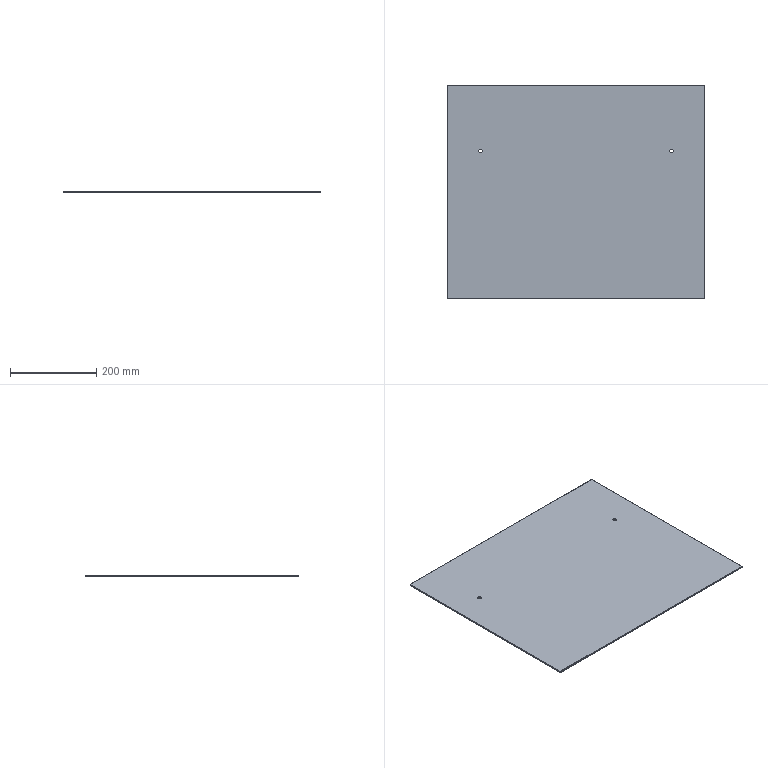Part | STEP file | ZXW722-L-05 | 1 solid | 22 faces | box 596 x 494 x 3 mm | volume 882649 mm3 | plane 10 | cylinder 8 | cone 4 | commonest cylinder face diameters 4 x4 8.5 x4
STEP:
#1=CARTESIAN_POINT('',(0.,0.,0.));
#2=DIRECTION('',(0.,0.,1.));
#3=DIRECTION('',(1.,0.,0.));
#4=AXIS2_PLACEMENT_3D('',#1,#2,#3);
#5=CARTESIAN_POINT('',(296.,245.5,0.000000011));
#6=VERTEX_POINT('',#5);
#7=CARTESIAN_POINT('',(-296.,245.5,0.));
#8=VERTEX_POINT('',#7);
#9=CARTESIAN_POINT('',(296.,245.5,0.000000011));
#10=DIRECTION('',(-1.,0.,0.));
#11=VECTOR('',#10,592.);
#12=LINE('',#9,#11);
#13=EDGE_CURVE('',#6,#8,#12,.T.);
#14=ORIENTED_EDGE('',*,*,#13,.F.);
#15=CARTESIAN_POINT('',(297.5,244.,0.));
#16=VERTEX_POINT('',#15);
#17=CARTESIAN_POINT('',(296.,244.,0.));
#18=DIRECTION('',(0.,0.,1.));
#19=DIRECTION('',(1.,0.,0.));
#20=AXIS2_PLACEMENT_3D('',#17,#18,#19);
#21=CIRCLE('',#20,1.5);
#22=EDGE_CURVE('',#16,#6,#21,.T.);
#23=ORIENTED_EDGE('',*,*,#22,.F.);
#24=CARTESIAN_POINT('',(297.5,-246.,0.));
#25=VERTEX_POINT('',#24);
#26=CARTESIAN_POINT('',(297.5,-246.,0.000000011));
#27=DIRECTION('',(0.,1.,0.));
#28=VECTOR('',#27,490.);
#29=LINE('',#26,#28);
#30=EDGE_CURVE('',#25,#16,#29,.T.);
#31=ORIENTED_EDGE('',*,*,#30,.F.);
#32=CARTESIAN_POINT('',(296.,-247.5,0.));
#33=VERTEX_POINT('',#32);
#34=CARTESIAN_POINT('',(296.,-246.,0.));
#35=DIRECTION('',(0.,0.,1.));
#36=DIRECTION('',(0.,-1.,0.));
#37=AXIS2_PLACEMENT_3D('',#34,#35,#36);
#38=CIRCLE('',#37,1.5);
#39=EDGE_CURVE('',#33,#25,#38,.T.);
#40=ORIENTED_EDGE('',*,*,#39,.F.);
#41=CARTESIAN_POINT('',(-296.,-247.5,0.));
#42=VERTEX_POINT('',#41);
#43=CARTESIAN_POINT('',(-296.,-247.5,0.000000011));
#44=DIRECTION('',(1.,0.,0.));
#45=VECTOR('',#44,592.);
#46=LINE('',#43,#45);
#47=EDGE_CURVE('',#42,#33,#46,.T.);
#48=ORIENTED_EDGE('',*,*,#47,.F.);
#49=CARTESIAN_POINT('',(-297.5,-246.,0.));
#50=VERTEX_POINT('',#49);
#51=CARTESIAN_POINT('',(-296.,-246.,0.));
#52=DIRECTION('',(0.,0.,1.));
#53=DIRECTION('',(-1.,0.,0.));
#54=AXIS2_PLACEMENT_3D('',#51,#52,#53);
#55=CIRCLE('',#54,1.5);
#56=EDGE_CURVE('',#50,#42,#55,.T.);
#57=ORIENTED_EDGE('',*,*,#56,.F.);
#58=CARTESIAN_POINT('',(-297.5,244.,0.));
#59=VERTEX_POINT('',#58);
#60=CARTESIAN_POINT('',(-297.5,244.,0.000000011));
#61=DIRECTION('',(0.,-1.,0.));
#62=VECTOR('',#61,490.);
#63=LINE('',#60,#62);
#64=EDGE_CURVE('',#59,#50,#63,.T.);
#65=ORIENTED_EDGE('',*,*,#64,.F.);
#66=CARTESIAN_POINT('',(-296.,244.,0.));
#67=DIRECTION('',(0.,0.,1.));
#68=DIRECTION('',(0.,1.,0.));
#69=AXIS2_PLACEMENT_3D('',#66,#67,#68);
#70=CIRCLE('',#69,1.5);
#71=EDGE_CURVE('',#8,#59,#70,.T.);
#72=ORIENTED_EDGE('',*,*,#71,.F.);
#73=EDGE_LOOP('',(#14,#23,#31,#40,#48,#57,#65,#72));
#74=FACE_OUTER_BOUND('',#73,.F.);
#75=CARTESIAN_POINT('',(-217.25,94.,0.));
#76=VERTEX_POINT('',#75);
#77=CARTESIAN_POINT('',(-225.75,94.,0.));
#78=VERTEX_POINT('',#77);
#79=CARTESIAN_POINT('',(-221.5,94.,0.));
#80=DIRECTION('',(0.,0.,1.));
#81=DIRECTION('',(1.,0.,0.));
#82=AXIS2_PLACEMENT_3D('',#79,#80,#81);
#83=CIRCLE('',#82,4.25);
#84=EDGE_CURVE('',#76,#78,#83,.T.);
#85=ORIENTED_EDGE('',*,*,#84,.T.);
#86=CARTESIAN_POINT('',(-221.5,94.,0.));
#87=DIRECTION('',(0.,0.,1.));
#88=DIRECTION('',(-1.,0.,0.));
#89=AXIS2_PLACEMENT_3D('',#86,#87,#88);
#90=CIRCLE('',#89,4.25);
#91=EDGE_CURVE('',#78,#76,#90,.T.);
#92=ORIENTED_EDGE('',*,*,#91,.T.);
#93=EDGE_LOOP('',(#85,#92));
#94=FACE_BOUND('',#93,.F.);
#95=CARTESIAN_POINT('',(225.75,94.,0.));
#96=VERTEX_POINT('',#95);
#97=CARTESIAN_POINT('',(217.25,94.,0.));
#98=VERTEX_POINT('',#97);
#99=CARTESIAN_POINT('',(221.5,94.,0.));
#100=DIRECTION('',(0.,0.,1.));
#101=DIRECTION('',(1.,0.,0.));
#102=AXIS2_PLACEMENT_3D('',#99,#100,#101);
#103=CIRCLE('',#102,4.25);
#104=EDGE_CURVE('',#96,#98,#103,.T.);
#105=ORIENTED_EDGE('',*,*,#104,.T.);
#106=CARTESIAN_POINT('',(221.5,94.,0.));
#107=DIRECTION('',(0.,0.,1.));
#108=DIRECTION('',(-1.,0.,0.));
#109=AXIS2_PLACEMENT_3D('',#106,#107,#108);
#110=CIRCLE('',#109,4.25);
#111=EDGE_CURVE('',#98,#96,#110,.T.);
#112=ORIENTED_EDGE('',*,*,#111,.T.);
#113=EDGE_LOOP('',(#105,#112));
#114=FACE_BOUND('',#113,.F.);
#115=CARTESIAN_POINT('',(0.,0.,0.));
#116=DIRECTION('',(0.,0.,1.));
#117=DIRECTION('',(1.,0.,0.));
#118=AXIS2_PLACEMENT_3D('',#115,#116,#117);
#119=PLANE('',#118);
#120=ADVANCED_FACE('',(#74,#94,#114),#119,.T.);
#121=ORIENTED_EDGE('',*,*,#13,.T.);
#122=CARTESIAN_POINT('',(-296.,246.,-0.5));
#123=VERTEX_POINT('',#122);
#124=CARTESIAN_POINT('',(-296.,245.5,0.));
#125=DIRECTION('',(0.,0.7071,-0.7071));
#126=VECTOR('',#125,0.7071);
#127=LINE('',#124,#126);
#128=EDGE_CURVE('',#8,#123,#127,.T.);
#129=ORIENTED_EDGE('',*,*,#128,.T.);
#130=CARTESIAN_POINT('',(296.,246.,-0.5));
#131=VERTEX_POINT('',#130);
#132=CARTESIAN_POINT('',(296.,246.,-0.5));
#133=DIRECTION('',(-1.,0.,0.));
#134=VECTOR('',#133,592.);
#135=LINE('',#132,#134);
#136=EDGE_CURVE('',#131,#123,#135,.T.);
#137=ORIENTED_EDGE('',*,*,#136,.F.);
#138=CARTESIAN_POINT('',(296.,245.5,0.000000011));
#139=DIRECTION('',(0.,0.7071,-0.7071));
#140=VECTOR('',#139,0.7071);
#141=LINE('',#138,#140);
#142=EDGE_CURVE('',#6,#131,#141,.T.);
#143=ORIENTED_EDGE('',*,*,#142,.F.);
#144=EDGE_LOOP('',(#121,#129,#137,#143));
#145=FACE_OUTER_BOUND('',#144,.F.);
#146=CARTESIAN_POINT('',(0.,245.75,-0.25));
#147=DIRECTION('',(0.,0.7071,0.7071));
#148=DIRECTION('',(0.,0.7071,-0.7071));
#149=AXIS2_PLACEMENT_3D('',#146,#147,#148);
#150=PLANE('',#149);
#151=ADVANCED_FACE('',(#145),#150,.T.);
#152=ORIENTED_EDGE('',*,*,#71,.T.);
#153=CARTESIAN_POINT('',(-298.,244.,-0.5));
#154=VERTEX_POINT('',#153);
#155=CARTESIAN_POINT('',(-297.5,244.,0.000000011));
#156=DIRECTION('',(-0.7071,0.,-0.7071));
#157=VECTOR('',#156,0.7071);
#158=LINE('',#155,#157);
#159=EDGE_CURVE('',#59,#154,#158,.T.);
#160=ORIENTED_EDGE('',*,*,#159,.T.);
#161=CARTESIAN_POINT('',(-296.,244.,-0.5));
#162=DIRECTION('',(0.,0.,1.));
#163=DIRECTION('',(0.,1.,0.));
#164=AXIS2_PLACEMENT_3D('',#161,#162,#163);
#165=CIRCLE('',#164,2.);
#166=EDGE_CURVE('',#123,#154,#165,.T.);
#167=ORIENTED_EDGE('',*,*,#166,.F.);
#168=ORIENTED_EDGE('',*,*,#128,.F.);
#169=EDGE_LOOP('',(#152,#160,#167,#168));
#170=FACE_OUTER_BOUND('',#169,.F.);
#171=CARTESIAN_POINT('',(-296.,244.,-0.25));
#172=DIRECTION('',(0.,0.,-1.));
#173=DIRECTION('',(0.,-1.,0.));
#174=AXIS2_PLACEMENT_3D('',#171,#172,#173);
#175=CONICAL_SURFACE('',#174,1.75,45.);
#176=ADVANCED_FACE('',(#170),#175,.T.);
#177=ORIENTED_EDGE('',*,*,#64,.T.);
#178=CARTESIAN_POINT('',(-298.,-246.,-0.5));
#179=VERTEX_POINT('',#178);
#180=CARTESIAN_POINT('',(-297.5,-246.,0.));
#181=DIRECTION('',(-0.7071,0.,-0.7071));
#182=VECTOR('',#181,0.7071);
#183=LINE('',#180,#182);
#184=EDGE_CURVE('',#50,#179,#183,.T.);
#185=ORIENTED_EDGE('',*,*,#184,.T.);
#186=CARTESIAN_POINT('',(-298.,244.,-0.5));
#187=DIRECTION('',(0.,-1.,0.));
#188=VECTOR('',#187,490.);
#189=LINE('',#186,#188);
#190=EDGE_CURVE('',#154,#179,#189,.T.);
#191=ORIENTED_EDGE('',*,*,#190,.F.);
#192=ORIENTED_EDGE('',*,*,#159,.F.);
#193=EDGE_LOOP('',(#177,#185,#191,#192));
#194=FACE_OUTER_BOUND('',#193,.F.);
#195=CARTESIAN_POINT('',(-297.75,-1.,-0.25));
#196=DIRECTION('',(-0.7071,0.,0.7071));
#197=DIRECTION('',(-0.7071,0.,-0.7071));
#198=AXIS2_PLACEMENT_3D('',#195,#196,#197);
#199=PLANE('',#198);
#200=ADVANCED_FACE('',(#194),#199,.T.);
#201=ORIENTED_EDGE('',*,*,#56,.T.);
#202=CARTESIAN_POINT('',(-296.,-248.,-0.5));
#203=VERTEX_POINT('',#202);
#204=CARTESIAN_POINT('',(-296.,-247.5,0.000000011));
#205=DIRECTION('',(0.,-0.7071,-0.7071));
#206=VECTOR('',#205,0.7071);
#207=LINE('',#204,#206);
#208=EDGE_CURVE('',#42,#203,#207,.T.);
#209=ORIENTED_EDGE('',*,*,#208,.T.);
#210=CARTESIAN_POINT('',(-296.,-246.,-0.5));
#211=DIRECTION('',(0.,0.,1.));
#212=DIRECTION('',(-1.,0.,0.));
#213=AXIS2_PLACEMENT_3D('',#210,#211,#212);
#214=CIRCLE('',#213,2.);
#215=EDGE_CURVE('',#179,#203,#214,.T.);
#216=ORIENTED_EDGE('',*,*,#215,.F.);
#217=ORIENTED_EDGE('',*,*,#184,.F.);
#218=EDGE_LOOP('',(#201,#209,#216,#217));
#219=FACE_OUTER_BOUND('',#218,.F.);
#220=CARTESIAN_POINT('',(-296.,-246.,-0.25));
#221=DIRECTION('',(0.,0.,-1.));
#222=DIRECTION('',(0.,-1.,0.));
#223=AXIS2_PLACEMENT_3D('',#220,#221,#222);
#224=CONICAL_SURFACE('',#223,1.75,45.);
#225=ADVANCED_FACE('',(#219),#224,.T.);
#226=ORIENTED_EDGE('',*,*,#47,.T.);
#227=CARTESIAN_POINT('',(296.,-248.,-0.5));
#228=VERTEX_POINT('',#227);
#229=CARTESIAN_POINT('',(296.,-247.5,0.));
#230=DIRECTION('',(0.,-0.7071,-0.7071));
#231=VECTOR('',#230,0.7071);
#232=LINE('',#229,#231);
#233=EDGE_CURVE('',#33,#228,#232,.T.);
#234=ORIENTED_EDGE('',*,*,#233,.T.);
#235=CARTESIAN_POINT('',(-296.,-248.,-0.5));
#236=DIRECTION('',(1.,0.,0.));
#237=VECTOR('',#236,592.);
#238=LINE('',#235,#237);
#239=EDGE_CURVE('',#203,#228,#238,.T.);
#240=ORIENTED_EDGE('',*,*,#239,.F.);
#241=ORIENTED_EDGE('',*,*,#208,.F.);
#242=EDGE_LOOP('',(#226,#234,#240,#241));
#243=FACE_OUTER_BOUND('',#242,.F.);
#244=CARTESIAN_POINT('',(0.,-247.75,-0.25));
#245=DIRECTION('',(0.,-0.7071,0.7071));
#246=DIRECTION('',(0.,-0.7071,-0.7071));
#247=AXIS2_PLACEMENT_3D('',#244,#245,#246);
#248=PLANE('',#247);
#249=ADVANCED_FACE('',(#243),#248,.T.);
#250=ORIENTED_EDGE('',*,*,#39,.T.);
#251=CARTESIAN_POINT('',(298.,-246.,-0.5));
#252=VERTEX_POINT('',#251);
#253=CARTESIAN_POINT('',(297.5,-246.,0.000000011));
#254=DIRECTION('',(0.7071,0.,-0.7071));
#255=VECTOR('',#254,0.7071);
#256=LINE('',#253,#255);
#257=EDGE_CURVE('',#25,#252,#256,.T.);
#258=ORIENTED_EDGE('',*,*,#257,.T.);
#259=CARTESIAN_POINT('',(296.,-246.,-0.5));
#260=DIRECTION('',(0.,0.,1.));
#261=DIRECTION('',(0.,-1.,0.));
#262=AXIS2_PLACEMENT_3D('',#259,#260,#261);
#263=CIRCLE('',#262,2.);
#264=EDGE_CURVE('',#228,#252,#263,.T.);
#265=ORIENTED_EDGE('',*,*,#264,.F.);
#266=ORIENTED_EDGE('',*,*,#233,.F.);
#267=EDGE_LOOP('',(#250,#258,#265,#266));
#268=FACE_OUTER_BOUND('',#267,.F.);
#269=CARTESIAN_POINT('',(296.,-246.,-0.25));
#270=DIRECTION('',(0.,0.,-1.));
#271=DIRECTION('',(0.,-1.,0.));
#272=AXIS2_PLACEMENT_3D('',#269,#270,#271);
#273=CONICAL_SURFACE('',#272,1.75,45.);
#274=ADVANCED_FACE('',(#268),#273,.T.);
#275=ORIENTED_EDGE('',*,*,#30,.T.);
#276=CARTESIAN_POINT('',(298.,244.,-0.5));
#277=VERTEX_POINT('',#276);
#278=CARTESIAN_POINT('',(297.5,244.,0.));
#279=DIRECTION('',(0.7071,0.,-0.7071));
#280=VECTOR('',#279,0.7071);
#281=LINE('',#278,#280);
#282=EDGE_CURVE('',#16,#277,#281,.T.);
#283=ORIENTED_EDGE('',*,*,#282,.T.);
#284=CARTESIAN_POINT('',(298.,-246.,-0.5));
#285=DIRECTION('',(0.,1.,0.));
#286=VECTOR('',#285,490.);
#287=LINE('',#284,#286);
#288=EDGE_CURVE('',#252,#277,#287,.T.);
#289=ORIENTED_EDGE('',*,*,#288,.F.);
#290=ORIENTED_EDGE('',*,*,#257,.F.);
#291=EDGE_LOOP('',(#275,#283,#289,#290));
#292=FACE_OUTER_BOUND('',#291,.F.);
#293=CARTESIAN_POINT('',(297.75,-1.,-0.25));
#294=DIRECTION('',(0.7071,0.,0.7071));
#295=DIRECTION('',(0.7071,0.,-0.7071));
#296=AXIS2_PLACEMENT_3D('',#293,#294,#295);
#297=PLANE('',#296);
#298=ADVANCED_FACE('',(#292),#297,.T.);
#299=ORIENTED_EDGE('',*,*,#142,.T.);
#300=CARTESIAN_POINT('',(296.,244.,-0.5));
#301=DIRECTION('',(0.,0.,1.));
#302=DIRECTION('',(1.,0.,0.));
#303=AXIS2_PLACEMENT_3D('',#300,#301,#302);
#304=CIRCLE('',#303,2.);
#305=EDGE_CURVE('',#277,#131,#304,.T.);
#306=ORIENTED_EDGE('',*,*,#305,.F.);
#307=ORIENTED_EDGE('',*,*,#282,.F.);
#308=ORIENTED_EDGE('',*,*,#22,.T.);
#309=EDGE_LOOP('',(#299,#306,#307,#308));
#310=FACE_OUTER_BOUND('',#309,.F.);
#311=CARTESIAN_POINT('',(296.,244.,-0.25));
#312=DIRECTION('',(0.,0.,-1.));
#313=DIRECTION('',(0.,-1.,0.));
#314=AXIS2_PLACEMENT_3D('',#311,#312,#313);
#315=CONICAL_SURFACE('',#314,1.75,45.);
#316=ADVANCED_FACE('',(#310),#315,.T.);
#317=ORIENTED_EDGE('',*,*,#305,.T.);
#318=CARTESIAN_POINT('',(296.,246.,-3.));
#319=VERTEX_POINT('',#318);
#320=CARTESIAN_POINT('',(296.,246.,-0.5));
#321=DIRECTION('',(-0.00000002,0.000000004,-1.));
#322=VECTOR('',#321,2.5);
#323=LINE('',#320,#322);
#324=EDGE_CURVE('',#131,#319,#323,.T.);
#325=ORIENTED_EDGE('',*,*,#324,.T.);
#326=CARTESIAN_POINT('',(298.,244.,-3.));
#327=VERTEX_POINT('',#326);
#328=CARTESIAN_POINT('',(296.,244.,-3.));
#329=DIRECTION('',(0.,0.,-1.));
#330=DIRECTION('',(0.,1.,0.));
#331=AXIS2_PLACEMENT_3D('',#328,#329,#330);
#332=CIRCLE('',#331,2.);
#333=EDGE_CURVE('',#319,#327,#332,.T.);
#334=ORIENTED_EDGE('',*,*,#333,.T.);
#335=CARTESIAN_POINT('',(298.,244.,-0.5));
#336=DIRECTION('',(0.,0.,-1.));
#337=VECTOR('',#336,2.5);
#338=LINE('',#335,#337);
#339=EDGE_CURVE('',#277,#327,#338,.T.);
#340=ORIENTED_EDGE('',*,*,#339,.F.);
#341=EDGE_LOOP('',(#317,#325,#334,#340));
#342=FACE_OUTER_BOUND('',#341,.F.);
#343=CARTESIAN_POINT('',(296.,244.,3.911));
#344=DIRECTION('',(0.,0.,-1.));
#345=DIRECTION('',(0.,1.,0.));
#346=AXIS2_PLACEMENT_3D('',#343,#344,#345);
#347=CYLINDRICAL_SURFACE('',#346,2.);
#348=ADVANCED_FACE('',(#342),#347,.T.);
#349=ORIENTED_EDGE('',*,*,#136,.T.);
#350=CARTESIAN_POINT('',(-296.,246.,-3.));
#351=VERTEX_POINT('',#350);
#352=CARTESIAN_POINT('',(-296.,246.,-0.5));
#353=DIRECTION('',(0.,0.,-1.));
#354=VECTOR('',#353,2.5);
#355=LINE('',#352,#354);
#356=EDGE_CURVE('',#123,#351,#355,.T.);
#357=ORIENTED_EDGE('',*,*,#356,.T.);
#358=CARTESIAN_POINT('',(296.,246.,-3.));
#359=DIRECTION('',(-1.,0.,0.));
#360=VECTOR('',#359,592.);
#361=LINE('',#358,#360);
#362=EDGE_CURVE('',#319,#351,#361,.T.);
#363=ORIENTED_EDGE('',*,*,#362,.F.);
#364=ORIENTED_EDGE('',*,*,#324,.F.);
#365=EDGE_LOOP('',(#349,#357,#363,#364));
#366=FACE_OUTER_BOUND('',#365,.F.);
#367=CARTESIAN_POINT('',(297.5,246.,0.));
#368=DIRECTION('',(0.,1.,0.));
#369=DIRECTION('',(-1.,0.,0.));
#370=AXIS2_PLACEMENT_3D('',#367,#368,#369);
#371=PLANE('',#370);
#372=ADVANCED_FACE('',(#366),#371,.T.);
#373=ORIENTED_EDGE('',*,*,#166,.T.);
#374=CARTESIAN_POINT('',(-298.,244.,-3.));
#375=VERTEX_POINT('',#374);
#376=CARTESIAN_POINT('',(-298.,244.,-0.5));
#377=DIRECTION('',(-0.000000004,-0.00000002,-1.));
#378=VECTOR('',#377,2.5);
#379=LINE('',#376,#378);
#380=EDGE_CURVE('',#154,#375,#379,.T.);
#381=ORIENTED_EDGE('',*,*,#380,.T.);
#382=CARTESIAN_POINT('',(-296.,244.,-3.));
#383=DIRECTION('',(0.,0.,-1.));
#384=DIRECTION('',(-1.,0.,0.));
#385=AXIS2_PLACEMENT_3D('',#382,#383,#384);
#386=CIRCLE('',#385,2.);
#387=EDGE_CURVE('',#375,#351,#386,.T.);
#388=ORIENTED_EDGE('',*,*,#387,.T.);
#389=ORIENTED_EDGE('',*,*,#356,.F.);
#390=EDGE_LOOP('',(#373,#381,#388,#389));
#391=FACE_OUTER_BOUND('',#390,.F.);
#392=CARTESIAN_POINT('',(-296.,244.,3.911));
#393=DIRECTION('',(0.,0.,-1.));
#394=DIRECTION('',(-1.,0.,0.));
#395=AXIS2_PLACEMENT_3D('',#392,#393,#394);
#396=CYLINDRICAL_SURFACE('',#395,2.);
#397=ADVANCED_FACE('',(#391),#396,.T.);
#398=ORIENTED_EDGE('',*,*,#190,.T.);
#399=CARTESIAN_POINT('',(-298.,-246.,-3.));
#400=VERTEX_POINT('',#399);
#401=CARTESIAN_POINT('',(-298.,-246.,-0.5));
#402=DIRECTION('',(0.,0.,-1.));
#403=VECTOR('',#402,2.5);
#404=LINE('',#401,#403);
#405=EDGE_CURVE('',#179,#400,#404,.T.);
#406=ORIENTED_EDGE('',*,*,#405,.T.);
#407=CARTESIAN_POINT('',(-298.,244.,-3.));
#408=DIRECTION('',(0.,-1.,0.));
#409=VECTOR('',#408,490.);
#410=LINE('',#407,#409);
#411=EDGE_CURVE('',#375,#400,#410,.T.);
#412=ORIENTED_EDGE('',*,*,#411,.F.);
#413=ORIENTED_EDGE('',*,*,#380,.F.);
#414=EDGE_LOOP('',(#398,#406,#412,#413));
#415=FACE_OUTER_BOUND('',#414,.F.);
#416=CARTESIAN_POINT('',(-298.,246.,0.));
#417=DIRECTION('',(-1.,0.,0.));
#418=DIRECTION('',(0.,-1.,0.));
#419=AXIS2_PLACEMENT_3D('',#416,#417,#418);
#420=PLANE('',#419);
#421=ADVANCED_FACE('',(#415),#420,.T.);
#422=ORIENTED_EDGE('',*,*,#215,.T.);
#423=CARTESIAN_POINT('',(-296.,-248.,-3.));
#424=VERTEX_POINT('',#423);
#425=CARTESIAN_POINT('',(-296.,-248.,-0.5));
#426=DIRECTION('',(0.00000002,-0.000000004,-1.));
#427=VECTOR('',#426,2.5);
#428=LINE('',#425,#427);
#429=EDGE_CURVE('',#203,#424,#428,.T.);
#430=ORIENTED_EDGE('',*,*,#429,.T.);
#431=CARTESIAN_POINT('',(-296.,-246.,-3.));
#432=DIRECTION('',(0.,0.,-1.));
#433=DIRECTION('',(0.,-1.,0.));
#434=AXIS2_PLACEMENT_3D('',#431,#432,#433);
#435=CIRCLE('',#434,2.);
#436=EDGE_CURVE('',#424,#400,#435,.T.);
#437=ORIENTED_EDGE('',*,*,#436,.T.);
#438=ORIENTED_EDGE('',*,*,#405,.F.);
#439=EDGE_LOOP('',(#422,#430,#437,#438));
#440=FACE_OUTER_BOUND('',#439,.F.);
#441=CARTESIAN_POINT('',(-296.,-246.,3.911));
#442=DIRECTION('',(0.,0.,-1.));
#443=DIRECTION('',(0.,-1.,0.));
#444=AXIS2_PLACEMENT_3D('',#441,#442,#443);
#445=CYLINDRICAL_SURFACE('',#444,2.);
#446=ADVANCED_FACE('',(#440),#445,.T.);
#447=ORIENTED_EDGE('',*,*,#239,.T.);
#448=CARTESIAN_POINT('',(296.,-248.,-3.));
#449=VERTEX_POINT('',#448);
#450=CARTESIAN_POINT('',(296.,-248.,-0.5));
#451=DIRECTION('',(0.,0.,-1.));
#452=VECTOR('',#451,2.5);
#453=LINE('',#450,#452);
#454=EDGE_CURVE('',#228,#449,#453,.T.);
#455=ORIENTED_EDGE('',*,*,#454,.T.);
#456=CARTESIAN_POINT('',(-296.,-248.,-3.));
#457=DIRECTION('',(1.,0.,0.));
#458=VECTOR('',#457,592.);
#459=LINE('',#456,#458);
#460=EDGE_CURVE('',#424,#449,#459,.T.);
#461=ORIENTED_EDGE('',*,*,#460,.F.);
#462=ORIENTED_EDGE('',*,*,#429,.F.);
#463=EDGE_LOOP('',(#447,#455,#461,#462));
#464=FACE_OUTER_BOUND('',#463,.F.);
#465=CARTESIAN_POINT('',(-297.5,-248.,0.));
#466=DIRECTION('',(0.,-1.,0.));
#467=DIRECTION('',(1.,0.,0.));
#468=AXIS2_PLACEMENT_3D('',#465,#466,#467);
#469=PLANE('',#468);
#470=ADVANCED_FACE('',(#464),#469,.T.);
#471=ORIENTED_EDGE('',*,*,#264,.T.);
#472=CARTESIAN_POINT('',(298.,-246.,-3.));
#473=VERTEX_POINT('',#472);
#474=CARTESIAN_POINT('',(298.,-246.,-0.5));
#475=DIRECTION('',(0.000000004,0.00000002,-1.));
#476=VECTOR('',#475,2.5);
#477=LINE('',#474,#476);
#478=EDGE_CURVE('',#252,#473,#477,.T.);
#479=ORIENTED_EDGE('',*,*,#478,.T.);
#480=CARTESIAN_POINT('',(296.,-246.,-3.));
#481=DIRECTION('',(0.,0.,-1.));
#482=DIRECTION('',(1.,0.,0.));
#483=AXIS2_PLACEMENT_3D('',#480,#481,#482);
#484=CIRCLE('',#483,2.);
#485=EDGE_CURVE('',#473,#449,#484,.T.);
#486=ORIENTED_EDGE('',*,*,#485,.T.);
#487=ORIENTED_EDGE('',*,*,#454,.F.);
#488=EDGE_LOOP('',(#471,#479,#486,#487));
#489=FACE_OUTER_BOUND('',#488,.F.);
#490=CARTESIAN_POINT('',(296.,-246.,3.911));
#491=DIRECTION('',(0.,0.,-1.));
#492=DIRECTION('',(1.,0.,0.));
#493=AXIS2_PLACEMENT_3D('',#490,#491,#492);
#494=CYLINDRICAL_SURFACE('',#493,2.);
#495=ADVANCED_FACE('',(#489),#494,.T.);
#496=ORIENTED_EDGE('',*,*,#288,.T.);
#497=ORIENTED_EDGE('',*,*,#339,.T.);
#498=CARTESIAN_POINT('',(298.,-246.,-3.));
#499=DIRECTION('',(0.,1.,0.));
#500=VECTOR('',#499,490.);
#501=LINE('',#498,#500);
#502=EDGE_CURVE('',#473,#327,#501,.T.);
#503=ORIENTED_EDGE('',*,*,#502,.F.);
#504=ORIENTED_EDGE('',*,*,#478,.F.);
#505=EDGE_LOOP('',(#496,#497,#503,#504));
#506=FACE_OUTER_BOUND('',#505,.F.);
#507=CARTESIAN_POINT('',(298.,-246.,0.));
#508=DIRECTION('',(1.,0.,0.));
#509=DIRECTION('',(0.,1.,0.));
#510=AXIS2_PLACEMENT_3D('',#507,#508,#509);
#511=PLANE('',#510);
#512=ADVANCED_FACE('',(#506),#511,.T.);
#513=ORIENTED_EDGE('',*,*,#333,.F.);
#514=ORIENTED_EDGE('',*,*,#362,.T.);
#515=ORIENTED_EDGE('',*,*,#387,.F.);
#516=ORIENTED_EDGE('',*,*,#411,.T.);
#517=ORIENTED_EDGE('',*,*,#436,.F.);
#518=ORIENTED_EDGE('',*,*,#460,.T.);
#519=ORIENTED_EDGE('',*,*,#485,.F.);
#520=ORIENTED_EDGE('',*,*,#502,.T.);
#521=EDGE_LOOP('',(#513,#514,#515,#516,#517,#518,#519,#520));
#522=FACE_OUTER_BOUND('',#521,.F.);
#523=CARTESIAN_POINT('',(-217.25,94.,-3.));
#524=VERTEX_POINT('',#523);
#525=CARTESIAN_POINT('',(-225.75,94.,-3.));
#526=VERTEX_POINT('',#525);
#527=CARTESIAN_POINT('',(-221.5,94.,-3.));
#528=DIRECTION('',(0.,0.,1.));
#529=DIRECTION('',(1.,0.,0.));
#530=AXIS2_PLACEMENT_3D('',#527,#528,#529);
#531=CIRCLE('',#530,4.25);
#532=EDGE_CURVE('',#524,#526,#531,.T.);
#533=ORIENTED_EDGE('',*,*,#532,.F.);
#534=CARTESIAN_POINT('',(-221.5,94.,-3.));
#535=DIRECTION('',(0.,0.,1.));
#536=DIRECTION('',(-1.,0.,0.));
#537=AXIS2_PLACEMENT_3D('',#534,#535,#536);
#538=CIRCLE('',#537,4.25);
#539=EDGE_CURVE('',#526,#524,#538,.T.);
#540=ORIENTED_EDGE('',*,*,#539,.F.);
#541=EDGE_LOOP('',(#533,#540));
#542=FACE_BOUND('',#541,.F.);
#543=CARTESIAN_POINT('',(225.75,94.,-3.));
#544=VERTEX_POINT('',#543);
#545=CARTESIAN_POINT('',(217.25,94.,-3.));
#546=VERTEX_POINT('',#545);
#547=CARTESIAN_POINT('',(221.5,94.,-3.));
#548=DIRECTION('',(0.,0.,1.));
#549=DIRECTION('',(1.,0.,0.));
#550=AXIS2_PLACEMENT_3D('',#547,#548,#549);
#551=CIRCLE('',#550,4.25);
#552=EDGE_CURVE('',#544,#546,#551,.T.);
#553=ORIENTED_EDGE('',*,*,#552,.F.);
#554=CARTESIAN_POINT('',(221.5,94.,-3.));
#555=DIRECTION('',(0.,0.,1.));
#556=DIRECTION('',(-1.,0.,0.));
#557=AXIS2_PLACEMENT_3D('',#554,#555,#556);
#558=CIRCLE('',#557,4.25);
#559=EDGE_CURVE('',#546,#544,#558,.T.);
#560=ORIENTED_EDGE('',*,*,#559,.F.);
#561=EDGE_LOOP('',(#553,#560));
#562=FACE_BOUND('',#561,.F.);
#563=CARTESIAN_POINT('',(0.,0.,-3.));
#564=DIRECTION('',(0.,0.,1.));
#565=DIRECTION('',(1.,0.,0.));
#566=AXIS2_PLACEMENT_3D('',#563,#564,#565);
#567=PLANE('',#566);
#568=ADVANCED_FACE('',(#522,#542,#562),#567,.F.);
#569=ORIENTED_EDGE('',*,*,#84,.F.);
#570=CARTESIAN_POINT('',(-217.25,94.,0.));
#571=DIRECTION('',(0.,0.,-1.));
#572=VECTOR('',#571,3.);
#573=LINE('',#570,#572);
#574=EDGE_CURVE('',#76,#524,#573,.T.);
#575=ORIENTED_EDGE('',*,*,#574,.T.);
#576=ORIENTED_EDGE('',*,*,#532,.T.);
#577=CARTESIAN_POINT('',(-225.75,94.,0.));
#578=DIRECTION('',(0.,0.,-1.));
#579=VECTOR('',#578,3.);
#580=LINE('',#577,#579);
#581=EDGE_CURVE('',#78,#526,#580,.T.);
#582=ORIENTED_EDGE('',*,*,#581,.F.);
#583=EDGE_LOOP('',(#569,#575,#576,#582));
#584=FACE_OUTER_BOUND('',#583,.F.);
#585=CARTESIAN_POINT('',(-221.5,94.,0.));
#586=DIRECTION('',(0.,0.,1.));
#587=DIRECTION('',(1.,0.,0.));
#588=AXIS2_PLACEMENT_3D('',#585,#586,#587);
#589=CYLINDRICAL_SURFACE('',#588,4.25);
#590=ADVANCED_FACE('',(#584),#589,.F.);
#591=ORIENTED_EDGE('',*,*,#91,.F.);
#592=ORIENTED_EDGE('',*,*,#581,.T.);
#593=ORIENTED_EDGE('',*,*,#539,.T.);
#594=ORIENTED_EDGE('',*,*,#574,.F.);
#595=EDGE_LOOP('',(#591,#592,#593,#594));
#596=FACE_OUTER_BOUND('',#595,.F.);
#597=CARTESIAN_POINT('',(-221.5,94.,0.));
#598=DIRECTION('',(0.,0.,1.));
#599=DIRECTION('',(1.,0.,0.));
#600=AXIS2_PLACEMENT_3D('',#597,#598,#599);
#601=CYLINDRICAL_SURFACE('',#600,4.25);
#602=ADVANCED_FACE('',(#596),#601,.F.);
#603=ORIENTED_EDGE('',*,*,#104,.F.);
#604=CARTESIAN_POINT('',(225.75,94.,0.));
#605=DIRECTION('',(0.,0.,-1.));
#606=VECTOR('',#605,3.);
#607=LINE('',#604,#606);
#608=EDGE_CURVE('',#96,#544,#607,.T.);
#609=ORIENTED_EDGE('',*,*,#608,.T.);
#610=ORIENTED_EDGE('',*,*,#552,.T.);
#611=CARTESIAN_POINT('',(217.25,94.,0.));
#612=DIRECTION('',(0.,0.,-1.));
#613=VECTOR('',#612,3.);
#614=LINE('',#611,#613);
#615=EDGE_CURVE('',#98,#546,#614,.T.);
#616=ORIENTED_EDGE('',*,*,#615,.F.);
#617=EDGE_LOOP('',(#603,#609,#610,#616));
#618=FACE_OUTER_BOUND('',#617,.F.);
#619=CARTESIAN_POINT('',(221.5,94.,0.));
#620=DIRECTION('',(0.,0.,1.));
#621=DIRECTION('',(1.,0.,0.));
#622=AXIS2_PLACEMENT_3D('',#619,#620,#621);
#623=CYLINDRICAL_SURFACE('',#622,4.25);
#624=ADVANCED_FACE('',(#618),#623,.F.);
#625=ORIENTED_EDGE('',*,*,#111,.F.);
#626=ORIENTED_EDGE('',*,*,#615,.T.);
#627=ORIENTED_EDGE('',*,*,#559,.T.);
#628=ORIENTED_EDGE('',*,*,#608,.F.);
#629=EDGE_LOOP('',(#625,#626,#627,#628));
#630=FACE_OUTER_BOUND('',#629,.F.);
#631=CARTESIAN_POINT('',(221.5,94.,0.));
#632=DIRECTION('',(0.,0.,1.));
#633=DIRECTION('',(1.,0.,0.));
#634=AXIS2_PLACEMENT_3D('',#631,#632,#633);
#635=CYLINDRICAL_SURFACE('',#634,4.25);
#636=ADVANCED_FACE('',(#630),#635,.F.);
#637=CLOSED_SHELL('',(#120,#151,#176,#200,#225,#249,#274,#298,#316,#348,#372,#397,#421,#446,#470,#495,#512,#568,#590,#602,#624,#636));
#638=MANIFOLD_SOLID_BREP('',#637);
#639=(LENGTH_UNIT()NAMED_UNIT(*)SI_UNIT(.MILLI.,.METRE.));
#640=UNCERTAINTY_MEASURE_WITH_UNIT(LENGTH_MEASURE(0.08492),#639,'','');
#641=(NAMED_UNIT(*)PLANE_ANGLE_UNIT()SI_UNIT($,.RADIAN.));
#642=PLANE_ANGLE_MEASURE_WITH_UNIT(PLANE_ANGLE_MEASURE(0.01745),#641);
#643=(CONVERSION_BASED_UNIT('DEGREE',#642)NAMED_UNIT(*)PLANE_ANGLE_UNIT());
#644=(NAMED_UNIT(*)SI_UNIT($,.STERADIAN.)SOLID_ANGLE_UNIT());
#645=(GEOMETRIC_REPRESENTATION_CONTEXT(3)GLOBAL_UNCERTAINTY_ASSIGNED_CONTEXT((#640))GLOBAL_UNIT_ASSIGNED_CONTEXT((#639,#643,#644))REPRESENTATION_CONTEXT('',''));
#646=ADVANCED_BREP_SHAPE_REPRESENTATION('',(#4,#638),#645);